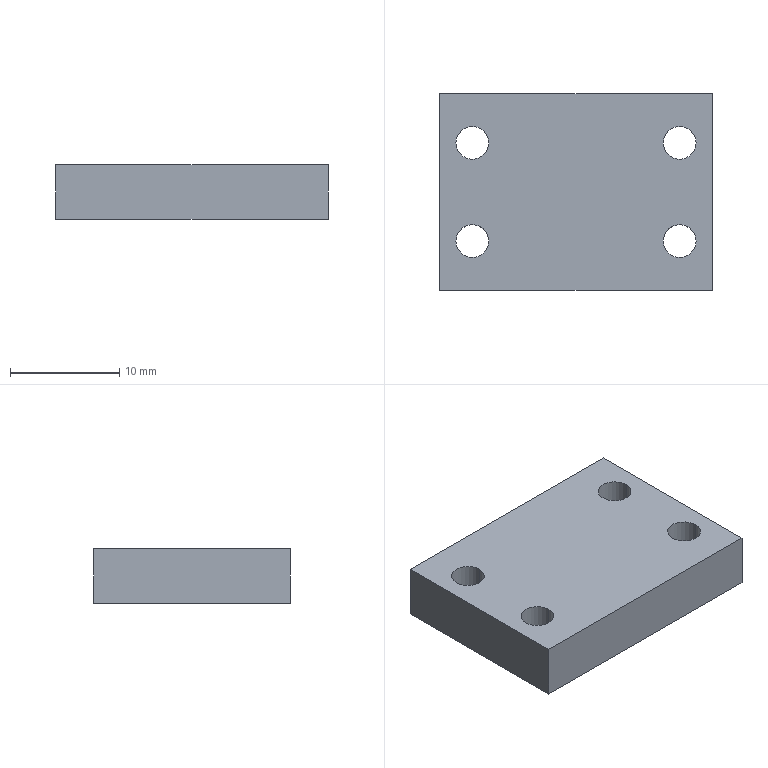Part | SolidWorks | features Extrusion 1 | 1 solid | 14 faces | box 25 x 18 x 5 mm | volume 2109 mm3 | cylinder 8 | plane 6 | commonest cylinder face diameters 3 x8
STEP:
#1=CARTESIAN_POINT('',(-11.,-4.5,5.));
#2=VERTEX_POINT('',#1);
#3=CARTESIAN_POINT('',(-8.,-4.5,5.));
#4=VERTEX_POINT('',#3);
#5=CARTESIAN_POINT('',(-9.5,-4.5,5.));
#6=DIRECTION('',(0.,0.,1.));
#7=DIRECTION('',(1.,0.,0.));
#8=AXIS2_PLACEMENT_3D('',#5,#6,#7);
#9=CIRCLE('',#8,1.5);
#10=EDGE_CURVE('',#2,#4,#9,.T.);
#11=ORIENTED_EDGE('',*,*,#10,.T.);
#12=CARTESIAN_POINT('',(-8.,-4.5,0.));
#13=VERTEX_POINT('',#12);
#14=CARTESIAN_POINT('',(-8.,-4.5,5.));
#15=DIRECTION('',(0.,0.,-1.));
#16=VECTOR('',#15,1000.);
#17=LINE('',#14,#16);
#18=EDGE_CURVE('',#4,#13,#17,.T.);
#19=ORIENTED_EDGE('',*,*,#18,.T.);
#20=CARTESIAN_POINT('',(-11.,-4.5,0.));
#21=VERTEX_POINT('',#20);
#22=CARTESIAN_POINT('',(-9.5,-4.5,0.));
#23=DIRECTION('',(0.,0.,1.));
#24=DIRECTION('',(1.,0.,0.));
#25=AXIS2_PLACEMENT_3D('',#22,#23,#24);
#26=CIRCLE('',#25,1.5);
#27=EDGE_CURVE('',#21,#13,#26,.T.);
#28=ORIENTED_EDGE('',*,*,#27,.F.);
#29=CARTESIAN_POINT('',(-11.,-4.5,5.));
#30=DIRECTION('',(0.,0.,-1.));
#31=VECTOR('',#30,1000.);
#32=LINE('',#29,#31);
#33=EDGE_CURVE('',#2,#21,#32,.T.);
#34=ORIENTED_EDGE('',*,*,#33,.F.);
#35=EDGE_LOOP('',(#11,#19,#28,#34));
#36=FACE_OUTER_BOUND('',#35,.T.);
#37=CARTESIAN_POINT('',(-9.5,-4.5,5.));
#38=DIRECTION('',(0.,0.,-1.));
#39=DIRECTION('',(-1.,0.,0.));
#40=AXIS2_PLACEMENT_3D('',#37,#38,#39);
#41=CYLINDRICAL_SURFACE('',#40,1.5);
#42=ADVANCED_FACE('',(#36),#41,.F.);
#43=CARTESIAN_POINT('',(8.,-4.5,5.));
#44=VERTEX_POINT('',#43);
#45=CARTESIAN_POINT('',(11.,-4.5,5.));
#46=VERTEX_POINT('',#45);
#47=CARTESIAN_POINT('',(9.5,-4.5,5.));
#48=DIRECTION('',(0.,0.,1.));
#49=DIRECTION('',(1.,0.,0.));
#50=AXIS2_PLACEMENT_3D('',#47,#48,#49);
#51=CIRCLE('',#50,1.5);
#52=EDGE_CURVE('',#44,#46,#51,.T.);
#53=ORIENTED_EDGE('',*,*,#52,.T.);
#54=CARTESIAN_POINT('',(11.,-4.5,0.));
#55=VERTEX_POINT('',#54);
#56=CARTESIAN_POINT('',(11.,-4.5,5.));
#57=DIRECTION('',(0.,0.,-1.));
#58=VECTOR('',#57,1000.);
#59=LINE('',#56,#58);
#60=EDGE_CURVE('',#46,#55,#59,.T.);
#61=ORIENTED_EDGE('',*,*,#60,.T.);
#62=CARTESIAN_POINT('',(8.,-4.5,0.));
#63=VERTEX_POINT('',#62);
#64=CARTESIAN_POINT('',(9.5,-4.5,0.));
#65=DIRECTION('',(0.,0.,1.));
#66=DIRECTION('',(1.,0.,0.));
#67=AXIS2_PLACEMENT_3D('',#64,#65,#66);
#68=CIRCLE('',#67,1.5);
#69=EDGE_CURVE('',#63,#55,#68,.T.);
#70=ORIENTED_EDGE('',*,*,#69,.F.);
#71=CARTESIAN_POINT('',(8.,-4.5,5.));
#72=DIRECTION('',(0.,0.,-1.));
#73=VECTOR('',#72,1000.);
#74=LINE('',#71,#73);
#75=EDGE_CURVE('',#44,#63,#74,.T.);
#76=ORIENTED_EDGE('',*,*,#75,.F.);
#77=EDGE_LOOP('',(#53,#61,#70,#76));
#78=FACE_OUTER_BOUND('',#77,.T.);
#79=CARTESIAN_POINT('',(9.5,-4.5,5.));
#80=DIRECTION('',(0.,0.,-1.));
#81=DIRECTION('',(-1.,0.,0.));
#82=AXIS2_PLACEMENT_3D('',#79,#80,#81);
#83=CYLINDRICAL_SURFACE('',#82,1.5);
#84=ADVANCED_FACE('',(#78),#83,.F.);
#85=CARTESIAN_POINT('',(8.,4.5,5.));
#86=VERTEX_POINT('',#85);
#87=CARTESIAN_POINT('',(11.,4.5,5.));
#88=VERTEX_POINT('',#87);
#89=CARTESIAN_POINT('',(9.5,4.5,5.));
#90=DIRECTION('',(0.,0.,1.));
#91=DIRECTION('',(1.,0.,0.));
#92=AXIS2_PLACEMENT_3D('',#89,#90,#91);
#93=CIRCLE('',#92,1.5);
#94=EDGE_CURVE('',#86,#88,#93,.T.);
#95=ORIENTED_EDGE('',*,*,#94,.T.);
#96=CARTESIAN_POINT('',(11.,4.5,0.));
#97=VERTEX_POINT('',#96);
#98=CARTESIAN_POINT('',(11.,4.5,5.));
#99=DIRECTION('',(0.,0.,-1.));
#100=VECTOR('',#99,1000.);
#101=LINE('',#98,#100);
#102=EDGE_CURVE('',#88,#97,#101,.T.);
#103=ORIENTED_EDGE('',*,*,#102,.T.);
#104=CARTESIAN_POINT('',(8.,4.5,0.));
#105=VERTEX_POINT('',#104);
#106=CARTESIAN_POINT('',(9.5,4.5,0.));
#107=DIRECTION('',(0.,0.,1.));
#108=DIRECTION('',(1.,0.,0.));
#109=AXIS2_PLACEMENT_3D('',#106,#107,#108);
#110=CIRCLE('',#109,1.5);
#111=EDGE_CURVE('',#105,#97,#110,.T.);
#112=ORIENTED_EDGE('',*,*,#111,.F.);
#113=CARTESIAN_POINT('',(8.,4.5,5.));
#114=DIRECTION('',(0.,0.,-1.));
#115=VECTOR('',#114,1000.);
#116=LINE('',#113,#115);
#117=EDGE_CURVE('',#86,#105,#116,.T.);
#118=ORIENTED_EDGE('',*,*,#117,.F.);
#119=EDGE_LOOP('',(#95,#103,#112,#118));
#120=FACE_OUTER_BOUND('',#119,.T.);
#121=CARTESIAN_POINT('',(9.5,4.5,5.));
#122=DIRECTION('',(0.,0.,-1.));
#123=DIRECTION('',(-1.,0.,0.));
#124=AXIS2_PLACEMENT_3D('',#121,#122,#123);
#125=CYLINDRICAL_SURFACE('',#124,1.5);
#126=ADVANCED_FACE('',(#120),#125,.F.);
#127=CARTESIAN_POINT('',(-11.,4.5,5.));
#128=VERTEX_POINT('',#127);
#129=CARTESIAN_POINT('',(-8.,4.5,5.));
#130=VERTEX_POINT('',#129);
#131=CARTESIAN_POINT('',(-9.5,4.5,5.));
#132=DIRECTION('',(0.,0.,1.));
#133=DIRECTION('',(1.,0.,0.));
#134=AXIS2_PLACEMENT_3D('',#131,#132,#133);
#135=CIRCLE('',#134,1.5);
#136=EDGE_CURVE('',#128,#130,#135,.T.);
#137=ORIENTED_EDGE('',*,*,#136,.T.);
#138=CARTESIAN_POINT('',(-8.,4.5,0.));
#139=VERTEX_POINT('',#138);
#140=CARTESIAN_POINT('',(-8.,4.5,5.));
#141=DIRECTION('',(0.,0.,-1.));
#142=VECTOR('',#141,1000.);
#143=LINE('',#140,#142);
#144=EDGE_CURVE('',#130,#139,#143,.T.);
#145=ORIENTED_EDGE('',*,*,#144,.T.);
#146=CARTESIAN_POINT('',(-11.,4.5,0.));
#147=VERTEX_POINT('',#146);
#148=CARTESIAN_POINT('',(-9.5,4.5,0.));
#149=DIRECTION('',(0.,0.,1.));
#150=DIRECTION('',(1.,0.,0.));
#151=AXIS2_PLACEMENT_3D('',#148,#149,#150);
#152=CIRCLE('',#151,1.5);
#153=EDGE_CURVE('',#147,#139,#152,.T.);
#154=ORIENTED_EDGE('',*,*,#153,.F.);
#155=CARTESIAN_POINT('',(-11.,4.5,5.));
#156=DIRECTION('',(0.,0.,-1.));
#157=VECTOR('',#156,1000.);
#158=LINE('',#155,#157);
#159=EDGE_CURVE('',#128,#147,#158,.T.);
#160=ORIENTED_EDGE('',*,*,#159,.F.);
#161=EDGE_LOOP('',(#137,#145,#154,#160));
#162=FACE_OUTER_BOUND('',#161,.T.);
#163=CARTESIAN_POINT('',(-9.5,4.5,5.));
#164=DIRECTION('',(0.,0.,-1.));
#165=DIRECTION('',(-1.,0.,0.));
#166=AXIS2_PLACEMENT_3D('',#163,#164,#165);
#167=CYLINDRICAL_SURFACE('',#166,1.5);
#168=ADVANCED_FACE('',(#162),#167,.F.);
#169=CARTESIAN_POINT('',(12.5,-9.,5.));
#170=VERTEX_POINT('',#169);
#171=CARTESIAN_POINT('',(12.5,9.,5.));
#172=VERTEX_POINT('',#171);
#173=CARTESIAN_POINT('',(12.5,-9.,5.));
#174=DIRECTION('',(0.,1.,0.));
#175=VECTOR('',#174,1000.);
#176=LINE('',#173,#175);
#177=EDGE_CURVE('',#170,#172,#176,.T.);
#178=ORIENTED_EDGE('',*,*,#177,.T.);
#179=CARTESIAN_POINT('',(-12.5,9.,5.));
#180=VERTEX_POINT('',#179);
#181=CARTESIAN_POINT('',(-12.5,9.,5.));
#182=DIRECTION('',(-1.,0.,0.));
#183=VECTOR('',#182,1000.);
#184=LINE('',#181,#183);
#185=EDGE_CURVE('',#172,#180,#184,.T.);
#186=ORIENTED_EDGE('',*,*,#185,.T.);
#187=CARTESIAN_POINT('',(-12.5,-9.,5.));
#188=VERTEX_POINT('',#187);
#189=CARTESIAN_POINT('',(-12.5,-9.,5.));
#190=DIRECTION('',(0.,-1.,0.));
#191=VECTOR('',#190,1000.);
#192=LINE('',#189,#191);
#193=EDGE_CURVE('',#180,#188,#192,.T.);
#194=ORIENTED_EDGE('',*,*,#193,.T.);
#195=CARTESIAN_POINT('',(-12.5,-9.,5.));
#196=DIRECTION('',(1.,0.,0.));
#197=VECTOR('',#196,1000.);
#198=LINE('',#195,#197);
#199=EDGE_CURVE('',#188,#170,#198,.T.);
#200=ORIENTED_EDGE('',*,*,#199,.T.);
#201=EDGE_LOOP('',(#178,#186,#194,#200));
#202=FACE_OUTER_BOUND('',#201,.T.);
#203=ORIENTED_EDGE('',*,*,#136,.F.);
#204=CARTESIAN_POINT('',(-9.5,4.5,5.));
#205=DIRECTION('',(0.,0.,1.));
#206=DIRECTION('',(1.,0.,0.));
#207=AXIS2_PLACEMENT_3D('',#204,#205,#206);
#208=CIRCLE('',#207,1.5);
#209=EDGE_CURVE('',#130,#128,#208,.T.);
#210=ORIENTED_EDGE('',*,*,#209,.F.);
#211=EDGE_LOOP('',(#203,#210));
#212=FACE_BOUND('',#211,.T.);
#213=ORIENTED_EDGE('',*,*,#94,.F.);
#214=CARTESIAN_POINT('',(9.5,4.5,5.));
#215=DIRECTION('',(0.,0.,1.));
#216=DIRECTION('',(1.,0.,0.));
#217=AXIS2_PLACEMENT_3D('',#214,#215,#216);
#218=CIRCLE('',#217,1.5);
#219=EDGE_CURVE('',#88,#86,#218,.T.);
#220=ORIENTED_EDGE('',*,*,#219,.F.);
#221=EDGE_LOOP('',(#213,#220));
#222=FACE_BOUND('',#221,.T.);
#223=ORIENTED_EDGE('',*,*,#52,.F.);
#224=CARTESIAN_POINT('',(9.5,-4.5,5.));
#225=DIRECTION('',(0.,0.,1.));
#226=DIRECTION('',(1.,0.,0.));
#227=AXIS2_PLACEMENT_3D('',#224,#225,#226);
#228=CIRCLE('',#227,1.5);
#229=EDGE_CURVE('',#46,#44,#228,.T.);
#230=ORIENTED_EDGE('',*,*,#229,.F.);
#231=EDGE_LOOP('',(#223,#230));
#232=FACE_BOUND('',#231,.T.);
#233=ORIENTED_EDGE('',*,*,#10,.F.);
#234=CARTESIAN_POINT('',(-9.5,-4.5,5.));
#235=DIRECTION('',(0.,0.,1.));
#236=DIRECTION('',(1.,0.,0.));
#237=AXIS2_PLACEMENT_3D('',#234,#235,#236);
#238=CIRCLE('',#237,1.5);
#239=EDGE_CURVE('',#4,#2,#238,.T.);
#240=ORIENTED_EDGE('',*,*,#239,.F.);
#241=EDGE_LOOP('',(#233,#240));
#242=FACE_BOUND('',#241,.T.);
#243=CARTESIAN_POINT('',(0.,0.,5.));
#244=DIRECTION('',(0.,0.,-1.));
#245=DIRECTION('',(-1.,0.,0.));
#246=AXIS2_PLACEMENT_3D('',#243,#244,#245);
#247=PLANE('',#246);
#248=ADVANCED_FACE('',(#202,#212,#222,#232,#242),#247,.F.);
#249=ORIENTED_EDGE('',*,*,#69,.T.);
#250=CARTESIAN_POINT('',(9.5,-4.5,0.));
#251=DIRECTION('',(0.,0.,1.));
#252=DIRECTION('',(1.,0.,0.));
#253=AXIS2_PLACEMENT_3D('',#250,#251,#252);
#254=CIRCLE('',#253,1.5);
#255=EDGE_CURVE('',#55,#63,#254,.T.);
#256=ORIENTED_EDGE('',*,*,#255,.T.);
#257=EDGE_LOOP('',(#249,#256));
#258=FACE_BOUND('',#257,.T.);
#259=ORIENTED_EDGE('',*,*,#153,.T.);
#260=CARTESIAN_POINT('',(-9.5,4.5,0.));
#261=DIRECTION('',(0.,0.,1.));
#262=DIRECTION('',(1.,0.,0.));
#263=AXIS2_PLACEMENT_3D('',#260,#261,#262);
#264=CIRCLE('',#263,1.5);
#265=EDGE_CURVE('',#139,#147,#264,.T.);
#266=ORIENTED_EDGE('',*,*,#265,.T.);
#267=EDGE_LOOP('',(#259,#266));
#268=FACE_BOUND('',#267,.T.);
#269=CARTESIAN_POINT('',(12.5,-9.,0.));
#270=VERTEX_POINT('',#269);
#271=CARTESIAN_POINT('',(12.5,9.,0.));
#272=VERTEX_POINT('',#271);
#273=CARTESIAN_POINT('',(12.5,-9.,0.));
#274=DIRECTION('',(0.,1.,0.));
#275=VECTOR('',#274,1000.);
#276=LINE('',#273,#275);
#277=EDGE_CURVE('',#270,#272,#276,.T.);
#278=ORIENTED_EDGE('',*,*,#277,.F.);
#279=CARTESIAN_POINT('',(-12.5,-9.,0.));
#280=VERTEX_POINT('',#279);
#281=CARTESIAN_POINT('',(-12.5,-9.,0.));
#282=DIRECTION('',(1.,0.,0.));
#283=VECTOR('',#282,1000.);
#284=LINE('',#281,#283);
#285=EDGE_CURVE('',#280,#270,#284,.T.);
#286=ORIENTED_EDGE('',*,*,#285,.F.);
#287=CARTESIAN_POINT('',(-12.5,9.,0.));
#288=VERTEX_POINT('',#287);
#289=CARTESIAN_POINT('',(-12.5,-9.,0.));
#290=DIRECTION('',(0.,-1.,0.));
#291=VECTOR('',#290,1000.);
#292=LINE('',#289,#291);
#293=EDGE_CURVE('',#288,#280,#292,.T.);
#294=ORIENTED_EDGE('',*,*,#293,.F.);
#295=CARTESIAN_POINT('',(-12.5,9.,0.));
#296=DIRECTION('',(-1.,0.,0.));
#297=VECTOR('',#296,1000.);
#298=LINE('',#295,#297);
#299=EDGE_CURVE('',#272,#288,#298,.T.);
#300=ORIENTED_EDGE('',*,*,#299,.F.);
#301=EDGE_LOOP('',(#278,#286,#294,#300));
#302=FACE_OUTER_BOUND('',#301,.T.);
#303=ORIENTED_EDGE('',*,*,#111,.T.);
#304=CARTESIAN_POINT('',(9.5,4.5,0.));
#305=DIRECTION('',(0.,0.,1.));
#306=DIRECTION('',(1.,0.,0.));
#307=AXIS2_PLACEMENT_3D('',#304,#305,#306);
#308=CIRCLE('',#307,1.5);
#309=EDGE_CURVE('',#97,#105,#308,.T.);
#310=ORIENTED_EDGE('',*,*,#309,.T.);
#311=EDGE_LOOP('',(#303,#310));
#312=FACE_BOUND('',#311,.T.);
#313=ORIENTED_EDGE('',*,*,#27,.T.);
#314=CARTESIAN_POINT('',(-9.5,-4.5,0.));
#315=DIRECTION('',(0.,0.,1.));
#316=DIRECTION('',(1.,0.,0.));
#317=AXIS2_PLACEMENT_3D('',#314,#315,#316);
#318=CIRCLE('',#317,1.5);
#319=EDGE_CURVE('',#13,#21,#318,.T.);
#320=ORIENTED_EDGE('',*,*,#319,.T.);
#321=EDGE_LOOP('',(#313,#320));
#322=FACE_BOUND('',#321,.T.);
#323=CARTESIAN_POINT('',(0.,0.,0.));
#324=DIRECTION('',(0.,0.,-1.));
#325=DIRECTION('',(-1.,0.,0.));
#326=AXIS2_PLACEMENT_3D('',#323,#324,#325);
#327=PLANE('',#326);
#328=ADVANCED_FACE('',(#258,#268,#302,#312,#322),#327,.T.);
#329=ORIENTED_EDGE('',*,*,#277,.T.);
#330=CARTESIAN_POINT('',(12.5,9.,5.));
#331=DIRECTION('',(0.,0.,-1.));
#332=VECTOR('',#331,1000.);
#333=LINE('',#330,#332);
#334=EDGE_CURVE('',#172,#272,#333,.T.);
#335=ORIENTED_EDGE('',*,*,#334,.F.);
#336=ORIENTED_EDGE('',*,*,#177,.F.);
#337=CARTESIAN_POINT('',(12.5,-9.,5.));
#338=DIRECTION('',(0.,0.,-1.));
#339=VECTOR('',#338,1000.);
#340=LINE('',#337,#339);
#341=EDGE_CURVE('',#170,#270,#340,.T.);
#342=ORIENTED_EDGE('',*,*,#341,.T.);
#343=EDGE_LOOP('',(#329,#335,#336,#342));
#344=FACE_OUTER_BOUND('',#343,.T.);
#345=CARTESIAN_POINT('',(12.5,-9.,5.));
#346=DIRECTION('',(-1.,0.,0.));
#347=DIRECTION('',(0.,0.,1.));
#348=AXIS2_PLACEMENT_3D('',#345,#346,#347);
#349=PLANE('',#348);
#350=ADVANCED_FACE('',(#344),#349,.F.);
#351=ORIENTED_EDGE('',*,*,#299,.T.);
#352=CARTESIAN_POINT('',(-12.5,9.,5.));
#353=DIRECTION('',(0.,0.,-1.));
#354=VECTOR('',#353,1000.);
#355=LINE('',#352,#354);
#356=EDGE_CURVE('',#180,#288,#355,.T.);
#357=ORIENTED_EDGE('',*,*,#356,.F.);
#358=ORIENTED_EDGE('',*,*,#185,.F.);
#359=ORIENTED_EDGE('',*,*,#334,.T.);
#360=EDGE_LOOP('',(#351,#357,#358,#359));
#361=FACE_OUTER_BOUND('',#360,.T.);
#362=CARTESIAN_POINT('',(-12.5,9.,5.));
#363=DIRECTION('',(0.,-1.,0.));
#364=DIRECTION('',(0.,0.,-1.));
#365=AXIS2_PLACEMENT_3D('',#362,#363,#364);
#366=PLANE('',#365);
#367=ADVANCED_FACE('',(#361),#366,.F.);
#368=ORIENTED_EDGE('',*,*,#293,.T.);
#369=CARTESIAN_POINT('',(-12.5,-9.,5.));
#370=DIRECTION('',(0.,0.,-1.));
#371=VECTOR('',#370,1000.);
#372=LINE('',#369,#371);
#373=EDGE_CURVE('',#188,#280,#372,.T.);
#374=ORIENTED_EDGE('',*,*,#373,.F.);
#375=ORIENTED_EDGE('',*,*,#193,.F.);
#376=ORIENTED_EDGE('',*,*,#356,.T.);
#377=EDGE_LOOP('',(#368,#374,#375,#376));
#378=FACE_OUTER_BOUND('',#377,.T.);
#379=CARTESIAN_POINT('',(-12.5,-9.,5.));
#380=DIRECTION('',(1.,0.,0.));
#381=DIRECTION('',(0.,0.,-1.));
#382=AXIS2_PLACEMENT_3D('',#379,#380,#381);
#383=PLANE('',#382);
#384=ADVANCED_FACE('',(#378),#383,.F.);
#385=ORIENTED_EDGE('',*,*,#285,.T.);
#386=ORIENTED_EDGE('',*,*,#341,.F.);
#387=ORIENTED_EDGE('',*,*,#199,.F.);
#388=ORIENTED_EDGE('',*,*,#373,.T.);
#389=EDGE_LOOP('',(#385,#386,#387,#388));
#390=FACE_OUTER_BOUND('',#389,.T.);
#391=CARTESIAN_POINT('',(-12.5,-9.,5.));
#392=DIRECTION('',(0.,1.,0.));
#393=DIRECTION('',(0.,0.,1.));
#394=AXIS2_PLACEMENT_3D('',#391,#392,#393);
#395=PLANE('',#394);
#396=ADVANCED_FACE('',(#390),#395,.F.);
#397=ORIENTED_EDGE('',*,*,#144,.F.);
#398=ORIENTED_EDGE('',*,*,#209,.T.);
#399=ORIENTED_EDGE('',*,*,#159,.T.);
#400=ORIENTED_EDGE('',*,*,#265,.F.);
#401=EDGE_LOOP('',(#397,#398,#399,#400));
#402=FACE_OUTER_BOUND('',#401,.T.);
#403=CARTESIAN_POINT('',(-9.5,4.5,5.));
#404=DIRECTION('',(0.,0.,-1.));
#405=DIRECTION('',(-1.,0.,0.));
#406=AXIS2_PLACEMENT_3D('',#403,#404,#405);
#407=CYLINDRICAL_SURFACE('',#406,1.5);
#408=ADVANCED_FACE('',(#402),#407,.F.);
#409=ORIENTED_EDGE('',*,*,#102,.F.);
#410=ORIENTED_EDGE('',*,*,#219,.T.);
#411=ORIENTED_EDGE('',*,*,#117,.T.);
#412=ORIENTED_EDGE('',*,*,#309,.F.);
#413=EDGE_LOOP('',(#409,#410,#411,#412));
#414=FACE_OUTER_BOUND('',#413,.T.);
#415=CARTESIAN_POINT('',(9.5,4.5,5.));
#416=DIRECTION('',(0.,0.,-1.));
#417=DIRECTION('',(-1.,0.,0.));
#418=AXIS2_PLACEMENT_3D('',#415,#416,#417);
#419=CYLINDRICAL_SURFACE('',#418,1.5);
#420=ADVANCED_FACE('',(#414),#419,.F.);
#421=ORIENTED_EDGE('',*,*,#60,.F.);
#422=ORIENTED_EDGE('',*,*,#229,.T.);
#423=ORIENTED_EDGE('',*,*,#75,.T.);
#424=ORIENTED_EDGE('',*,*,#255,.F.);
#425=EDGE_LOOP('',(#421,#422,#423,#424));
#426=FACE_OUTER_BOUND('',#425,.T.);
#427=CARTESIAN_POINT('',(9.5,-4.5,5.));
#428=DIRECTION('',(0.,0.,-1.));
#429=DIRECTION('',(-1.,0.,0.));
#430=AXIS2_PLACEMENT_3D('',#427,#428,#429);
#431=CYLINDRICAL_SURFACE('',#430,1.5);
#432=ADVANCED_FACE('',(#426),#431,.F.);
#433=ORIENTED_EDGE('',*,*,#18,.F.);
#434=ORIENTED_EDGE('',*,*,#239,.T.);
#435=ORIENTED_EDGE('',*,*,#33,.T.);
#436=ORIENTED_EDGE('',*,*,#319,.F.);
#437=EDGE_LOOP('',(#433,#434,#435,#436));
#438=FACE_OUTER_BOUND('',#437,.T.);
#439=CARTESIAN_POINT('',(-9.5,-4.5,5.));
#440=DIRECTION('',(0.,0.,-1.));
#441=DIRECTION('',(-1.,0.,0.));
#442=AXIS2_PLACEMENT_3D('',#439,#440,#441);
#443=CYLINDRICAL_SURFACE('',#442,1.5);
#444=ADVANCED_FACE('',(#438),#443,.F.);
#445=CLOSED_SHELL('',(#42,#84,#126,#168,#248,#328,#350,#367,#384,#396,#408,#420,#432,#444));
#446=MANIFOLD_SOLID_BREP('',#445);
#447=CARTESIAN_POINT('',(0.,0.,0.));
#448=DIRECTION('',(0.,0.,1.));
#449=DIRECTION('',(1.,0.,0.));
#450=AXIS2_PLACEMENT_3D('',#447,#448,#449);
#451=(LENGTH_UNIT()NAMED_UNIT(*)SI_UNIT(.MILLI.,.METRE.));
#452=UNCERTAINTY_MEASURE_WITH_UNIT(LENGTH_MEASURE(0.00001),#451,'','');
#453=(NAMED_UNIT(*)PLANE_ANGLE_UNIT()SI_UNIT($,.RADIAN.));
#454=(NAMED_UNIT(*)SI_UNIT($,.STERADIAN.)SOLID_ANGLE_UNIT());
#455=(GEOMETRIC_REPRESENTATION_CONTEXT(3)GLOBAL_UNCERTAINTY_ASSIGNED_CONTEXT((#452))GLOBAL_UNIT_ASSIGNED_CONTEXT((#451,#453,#454))REPRESENTATION_CONTEXT('',''));
#456=ADVANCED_BREP_SHAPE_REPRESENTATION('',(#446,#450),#455);